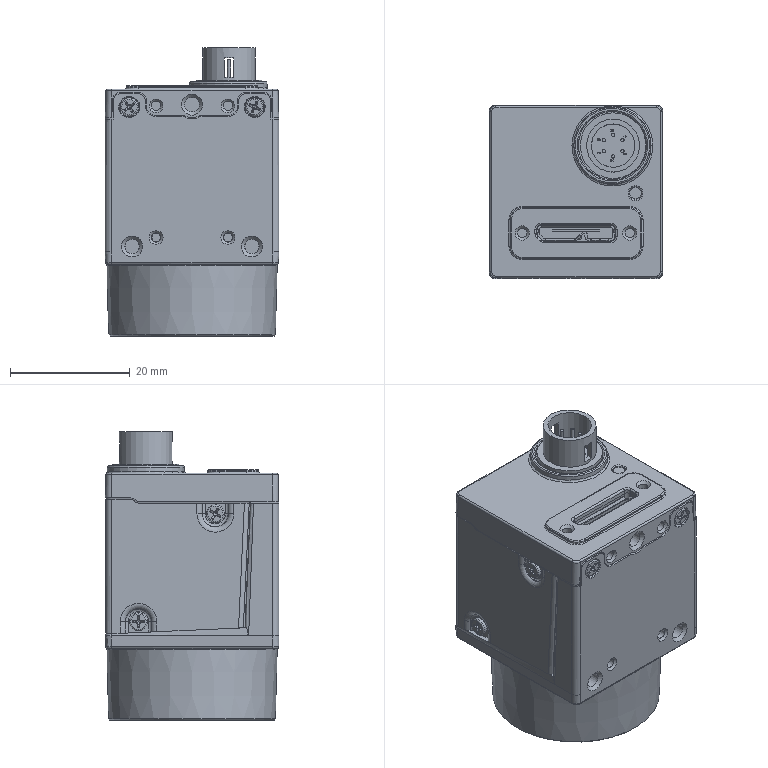Part | STEP file | Basler ace USB3 C-Mount v02-1-1_17 | 1 solid | 924 faces | box 29 x 29 x 48.2 mm | volume 25313 mm3 | plane 486 | cylinder 160 | cone 112 | spline 90 | torus 76 | commonest cylinder face diameters 2 x28 0.4 x22 0.6 x20 0.2 x14 1 x8 0.7 x7